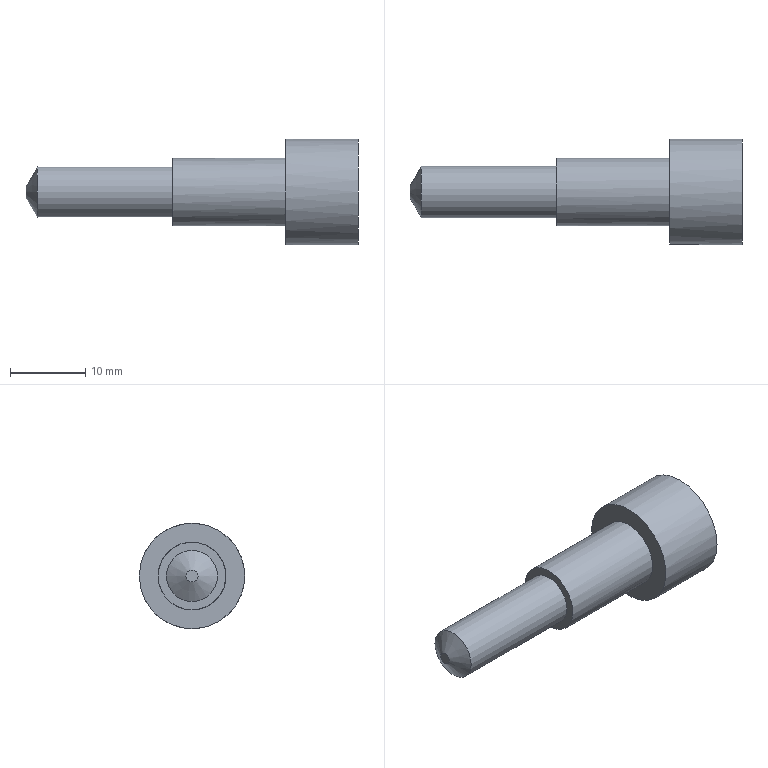Part | STEP file | solid 251 | 1 solid | 8 faces | box 44.094 x 14 x 14 mm | volume 3108 mm3 | plane 4 | cylinder 3 | cone 1 | commonest cylinder face diameters 6.8 x1 9 x1 14 x1